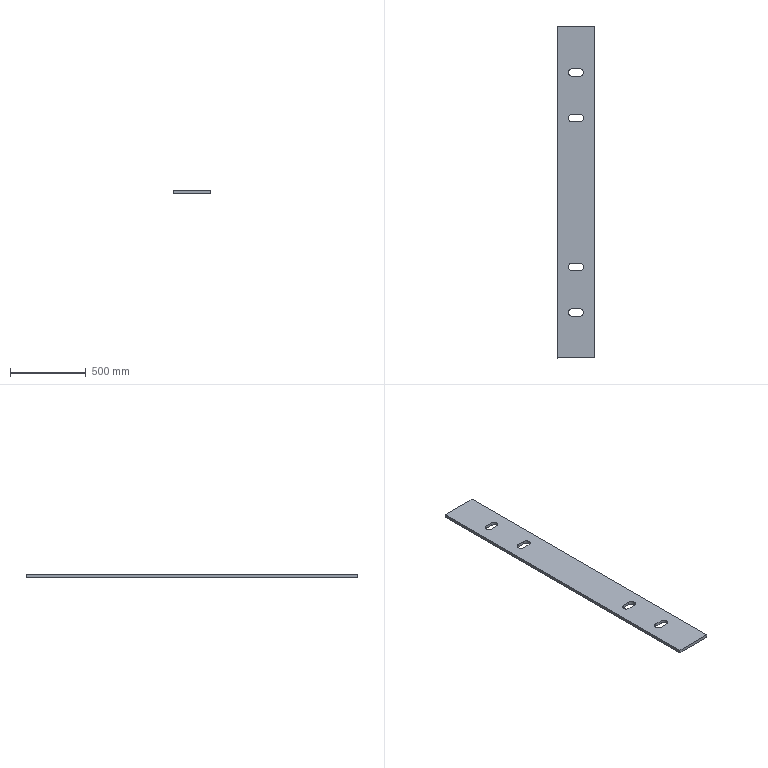Part | SolidWorks | features Extrusion 1 | 1 solid | 26 faces | box 250 x 2186 x 20 mm | volume 10572920 mm3 | plane 14 | cylinder 12 | commonest cylinder face diameters 50 x12
STEP:
#1=CARTESIAN_POINT('',(7508.99,4367.986,20.));
#2=VERTEX_POINT('',#1);
#3=CARTESIAN_POINT('',(7483.99,4342.986,20.));
#4=VERTEX_POINT('',#3);
#5=CARTESIAN_POINT('',(7508.99,4342.986,20.));
#6=DIRECTION('',(0.,0.,1.));
#7=DIRECTION('',(1.,0.,0.));
#8=AXIS2_PLACEMENT_3D('',#5,#6,#7);
#9=CIRCLE('',#8,25.);
#10=EDGE_CURVE('',#2,#4,#9,.T.);
#11=ORIENTED_EDGE('',*,*,#10,.T.);
#12=CARTESIAN_POINT('',(7483.99,4342.986,0.));
#13=VERTEX_POINT('',#12);
#14=CARTESIAN_POINT('',(7483.99,4342.986,20.));
#15=DIRECTION('',(0.,0.,-1.));
#16=VECTOR('',#15,1000.);
#17=LINE('',#14,#16);
#18=EDGE_CURVE('',#4,#13,#17,.T.);
#19=ORIENTED_EDGE('',*,*,#18,.T.);
#20=CARTESIAN_POINT('',(7508.99,4367.986,0.));
#21=VERTEX_POINT('',#20);
#22=CARTESIAN_POINT('',(7508.99,4342.986,0.));
#23=DIRECTION('',(0.,0.,1.));
#24=DIRECTION('',(1.,0.,0.));
#25=AXIS2_PLACEMENT_3D('',#22,#23,#24);
#26=CIRCLE('',#25,25.);
#27=EDGE_CURVE('',#21,#13,#26,.T.);
#28=ORIENTED_EDGE('',*,*,#27,.F.);
#29=CARTESIAN_POINT('',(7508.99,4367.986,20.));
#30=DIRECTION('',(0.,0.,-1.));
#31=VECTOR('',#30,1000.);
#32=LINE('',#29,#31);
#33=EDGE_CURVE('',#2,#21,#32,.T.);
#34=ORIENTED_EDGE('',*,*,#33,.F.);
#35=EDGE_LOOP('',(#11,#19,#28,#34));
#36=FACE_OUTER_BOUND('',#35,.T.);
#37=CARTESIAN_POINT('',(7508.99,4342.986,20.));
#38=DIRECTION('',(0.,0.,-1.));
#39=DIRECTION('',(-1.,0.,0.));
#40=AXIS2_PLACEMENT_3D('',#37,#38,#39);
#41=CYLINDRICAL_SURFACE('',#40,25.);
#42=ADVANCED_FACE('',(#36),#41,.F.);
#43=CARTESIAN_POINT('',(7508.99,4067.986,20.));
#44=VERTEX_POINT('',#43);
#45=CARTESIAN_POINT('',(7483.99,4042.986,20.));
#46=VERTEX_POINT('',#45);
#47=CARTESIAN_POINT('',(7508.99,4042.986,20.));
#48=DIRECTION('',(0.,0.,1.));
#49=DIRECTION('',(1.,0.,0.));
#50=AXIS2_PLACEMENT_3D('',#47,#48,#49);
#51=CIRCLE('',#50,25.);
#52=EDGE_CURVE('',#44,#46,#51,.T.);
#53=ORIENTED_EDGE('',*,*,#52,.T.);
#54=CARTESIAN_POINT('',(7483.99,4042.986,0.));
#55=VERTEX_POINT('',#54);
#56=CARTESIAN_POINT('',(7483.99,4042.986,20.));
#57=DIRECTION('',(0.,0.,-1.));
#58=VECTOR('',#57,1000.);
#59=LINE('',#56,#58);
#60=EDGE_CURVE('',#46,#55,#59,.T.);
#61=ORIENTED_EDGE('',*,*,#60,.T.);
#62=CARTESIAN_POINT('',(7508.99,4067.986,0.));
#63=VERTEX_POINT('',#62);
#64=CARTESIAN_POINT('',(7508.99,4042.986,0.));
#65=DIRECTION('',(0.,0.,1.));
#66=DIRECTION('',(1.,0.,0.));
#67=AXIS2_PLACEMENT_3D('',#64,#65,#66);
#68=CIRCLE('',#67,25.);
#69=EDGE_CURVE('',#63,#55,#68,.T.);
#70=ORIENTED_EDGE('',*,*,#69,.F.);
#71=CARTESIAN_POINT('',(7508.99,4067.986,20.));
#72=DIRECTION('',(0.,0.,-1.));
#73=VECTOR('',#72,1000.);
#74=LINE('',#71,#73);
#75=EDGE_CURVE('',#44,#63,#74,.T.);
#76=ORIENTED_EDGE('',*,*,#75,.F.);
#77=EDGE_LOOP('',(#53,#61,#70,#76));
#78=FACE_OUTER_BOUND('',#77,.T.);
#79=CARTESIAN_POINT('',(7508.99,4042.986,20.));
#80=DIRECTION('',(0.,0.,-1.));
#81=DIRECTION('',(-1.,0.,0.));
#82=AXIS2_PLACEMENT_3D('',#79,#80,#81);
#83=CYLINDRICAL_SURFACE('',#82,25.);
#84=ADVANCED_FACE('',(#78),#83,.F.);
#85=CARTESIAN_POINT('',(7508.99,3087.986,20.));
#86=VERTEX_POINT('',#85);
#87=CARTESIAN_POINT('',(7483.99,3062.986,20.));
#88=VERTEX_POINT('',#87);
#89=CARTESIAN_POINT('',(7508.99,3062.986,20.));
#90=DIRECTION('',(0.,0.,1.));
#91=DIRECTION('',(1.,0.,0.));
#92=AXIS2_PLACEMENT_3D('',#89,#90,#91);
#93=CIRCLE('',#92,25.);
#94=EDGE_CURVE('',#86,#88,#93,.T.);
#95=ORIENTED_EDGE('',*,*,#94,.T.);
#96=CARTESIAN_POINT('',(7483.99,3062.986,0.));
#97=VERTEX_POINT('',#96);
#98=CARTESIAN_POINT('',(7483.99,3062.986,20.));
#99=DIRECTION('',(0.,0.,-1.));
#100=VECTOR('',#99,1000.);
#101=LINE('',#98,#100);
#102=EDGE_CURVE('',#88,#97,#101,.T.);
#103=ORIENTED_EDGE('',*,*,#102,.T.);
#104=CARTESIAN_POINT('',(7508.99,3087.986,0.));
#105=VERTEX_POINT('',#104);
#106=CARTESIAN_POINT('',(7508.99,3062.986,0.));
#107=DIRECTION('',(0.,0.,1.));
#108=DIRECTION('',(1.,0.,0.));
#109=AXIS2_PLACEMENT_3D('',#106,#107,#108);
#110=CIRCLE('',#109,25.);
#111=EDGE_CURVE('',#105,#97,#110,.T.);
#112=ORIENTED_EDGE('',*,*,#111,.F.);
#113=CARTESIAN_POINT('',(7508.99,3087.986,20.));
#114=DIRECTION('',(0.,0.,-1.));
#115=VECTOR('',#114,1000.);
#116=LINE('',#113,#115);
#117=EDGE_CURVE('',#86,#105,#116,.T.);
#118=ORIENTED_EDGE('',*,*,#117,.F.);
#119=EDGE_LOOP('',(#95,#103,#112,#118));
#120=FACE_OUTER_BOUND('',#119,.T.);
#121=CARTESIAN_POINT('',(7508.99,3062.986,20.));
#122=DIRECTION('',(0.,0.,-1.));
#123=DIRECTION('',(-1.,0.,0.));
#124=AXIS2_PLACEMENT_3D('',#121,#122,#123);
#125=CYLINDRICAL_SURFACE('',#124,25.);
#126=ADVANCED_FACE('',(#120),#125,.F.);
#127=CARTESIAN_POINT('',(7508.99,2787.986,20.));
#128=VERTEX_POINT('',#127);
#129=CARTESIAN_POINT('',(7483.99,2762.986,20.));
#130=VERTEX_POINT('',#129);
#131=CARTESIAN_POINT('',(7508.99,2762.986,20.));
#132=DIRECTION('',(0.,0.,1.));
#133=DIRECTION('',(1.,0.,0.));
#134=AXIS2_PLACEMENT_3D('',#131,#132,#133);
#135=CIRCLE('',#134,25.);
#136=EDGE_CURVE('',#128,#130,#135,.T.);
#137=ORIENTED_EDGE('',*,*,#136,.T.);
#138=CARTESIAN_POINT('',(7483.99,2762.986,0.));
#139=VERTEX_POINT('',#138);
#140=CARTESIAN_POINT('',(7483.99,2762.986,20.));
#141=DIRECTION('',(0.,0.,-1.));
#142=VECTOR('',#141,1000.);
#143=LINE('',#140,#142);
#144=EDGE_CURVE('',#130,#139,#143,.T.);
#145=ORIENTED_EDGE('',*,*,#144,.T.);
#146=CARTESIAN_POINT('',(7508.99,2787.986,0.));
#147=VERTEX_POINT('',#146);
#148=CARTESIAN_POINT('',(7508.99,2762.986,0.));
#149=DIRECTION('',(0.,0.,1.));
#150=DIRECTION('',(1.,0.,0.));
#151=AXIS2_PLACEMENT_3D('',#148,#149,#150);
#152=CIRCLE('',#151,25.);
#153=EDGE_CURVE('',#147,#139,#152,.T.);
#154=ORIENTED_EDGE('',*,*,#153,.F.);
#155=CARTESIAN_POINT('',(7508.99,2787.986,20.));
#156=DIRECTION('',(0.,0.,-1.));
#157=VECTOR('',#156,1000.);
#158=LINE('',#155,#157);
#159=EDGE_CURVE('',#128,#147,#158,.T.);
#160=ORIENTED_EDGE('',*,*,#159,.F.);
#161=EDGE_LOOP('',(#137,#145,#154,#160));
#162=FACE_OUTER_BOUND('',#161,.T.);
#163=CARTESIAN_POINT('',(7508.99,2762.986,20.));
#164=DIRECTION('',(0.,0.,-1.));
#165=DIRECTION('',(-1.,0.,0.));
#166=AXIS2_PLACEMENT_3D('',#163,#164,#165);
#167=CYLINDRICAL_SURFACE('',#166,25.);
#168=ADVANCED_FACE('',(#162),#167,.F.);
#169=CARTESIAN_POINT('',(7408.99,2462.986,20.));
#170=VERTEX_POINT('',#169);
#171=CARTESIAN_POINT('',(7658.99,2462.986,20.));
#172=VERTEX_POINT('',#171);
#173=CARTESIAN_POINT('',(7408.99,2462.986,20.));
#174=DIRECTION('',(1.,0.,0.));
#175=VECTOR('',#174,1000.);
#176=LINE('',#173,#175);
#177=EDGE_CURVE('',#170,#172,#176,.T.);
#178=ORIENTED_EDGE('',*,*,#177,.T.);
#179=CARTESIAN_POINT('',(7658.99,4648.986,20.));
#180=VERTEX_POINT('',#179);
#181=CARTESIAN_POINT('',(7658.99,2462.986,20.));
#182=DIRECTION('',(0.,1.,0.));
#183=VECTOR('',#182,1000.);
#184=LINE('',#181,#183);
#185=EDGE_CURVE('',#172,#180,#184,.T.);
#186=ORIENTED_EDGE('',*,*,#185,.T.);
#187=CARTESIAN_POINT('',(7408.99,4648.986,20.));
#188=VERTEX_POINT('',#187);
#189=CARTESIAN_POINT('',(7408.99,4648.986,20.));
#190=DIRECTION('',(-1.,0.,0.));
#191=VECTOR('',#190,1000.);
#192=LINE('',#189,#191);
#193=EDGE_CURVE('',#180,#188,#192,.T.);
#194=ORIENTED_EDGE('',*,*,#193,.T.);
#195=CARTESIAN_POINT('',(7408.99,2462.986,20.));
#196=DIRECTION('',(0.,-1.,0.));
#197=VECTOR('',#196,1000.);
#198=LINE('',#195,#197);
#199=EDGE_CURVE('',#188,#170,#198,.T.);
#200=ORIENTED_EDGE('',*,*,#199,.T.);
#201=EDGE_LOOP('',(#178,#186,#194,#200));
#202=FACE_OUTER_BOUND('',#201,.T.);
#203=CARTESIAN_POINT('',(7508.99,2737.986,20.));
#204=VERTEX_POINT('',#203);
#205=CARTESIAN_POINT('',(7558.99,2737.986,20.));
#206=VERTEX_POINT('',#205);
#207=CARTESIAN_POINT('',(7508.99,2737.986,20.));
#208=DIRECTION('',(1.,0.,0.));
#209=VECTOR('',#208,1000.);
#210=LINE('',#207,#209);
#211=EDGE_CURVE('',#204,#206,#210,.T.);
#212=ORIENTED_EDGE('',*,*,#211,.F.);
#213=CARTESIAN_POINT('',(7508.99,2762.986,20.));
#214=DIRECTION('',(0.,0.,1.));
#215=DIRECTION('',(1.,0.,0.));
#216=AXIS2_PLACEMENT_3D('',#213,#214,#215);
#217=CIRCLE('',#216,25.);
#218=EDGE_CURVE('',#130,#204,#217,.T.);
#219=ORIENTED_EDGE('',*,*,#218,.F.);
#220=ORIENTED_EDGE('',*,*,#136,.F.);
#221=CARTESIAN_POINT('',(7558.989,2787.986,20.));
#222=VERTEX_POINT('',#221);
#223=CARTESIAN_POINT('',(7508.99,2787.986,20.));
#224=DIRECTION('',(-1.,0.,0.));
#225=VECTOR('',#224,1000.);
#226=LINE('',#223,#225);
#227=EDGE_CURVE('',#222,#128,#226,.T.);
#228=ORIENTED_EDGE('',*,*,#227,.F.);
#229=CARTESIAN_POINT('',(7558.99,2762.986,20.));
#230=DIRECTION('',(0.,0.,1.));
#231=DIRECTION('',(1.,0.,0.));
#232=AXIS2_PLACEMENT_3D('',#229,#230,#231);
#233=CIRCLE('',#232,25.);
#234=EDGE_CURVE('',#206,#222,#233,.T.);
#235=ORIENTED_EDGE('',*,*,#234,.F.);
#236=EDGE_LOOP('',(#212,#219,#220,#228,#235));
#237=FACE_BOUND('',#236,.T.);
#238=CARTESIAN_POINT('',(7508.99,3037.986,20.));
#239=VERTEX_POINT('',#238);
#240=CARTESIAN_POINT('',(7558.99,3037.986,20.));
#241=VERTEX_POINT('',#240);
#242=CARTESIAN_POINT('',(7558.99,3037.986,20.));
#243=DIRECTION('',(1.,0.,0.));
#244=VECTOR('',#243,1000.);
#245=LINE('',#242,#244);
#246=EDGE_CURVE('',#239,#241,#245,.T.);
#247=ORIENTED_EDGE('',*,*,#246,.F.);
#248=CARTESIAN_POINT('',(7508.99,3062.986,20.));
#249=DIRECTION('',(0.,0.,1.));
#250=DIRECTION('',(1.,0.,0.));
#251=AXIS2_PLACEMENT_3D('',#248,#249,#250);
#252=CIRCLE('',#251,25.);
#253=EDGE_CURVE('',#88,#239,#252,.T.);
#254=ORIENTED_EDGE('',*,*,#253,.F.);
#255=ORIENTED_EDGE('',*,*,#94,.F.);
#256=CARTESIAN_POINT('',(7558.989,3087.986,20.));
#257=VERTEX_POINT('',#256);
#258=CARTESIAN_POINT('',(7508.99,3087.986,20.));
#259=DIRECTION('',(-1.,0.,0.));
#260=VECTOR('',#259,1000.);
#261=LINE('',#258,#260);
#262=EDGE_CURVE('',#257,#86,#261,.T.);
#263=ORIENTED_EDGE('',*,*,#262,.F.);
#264=CARTESIAN_POINT('',(7558.99,3062.986,20.));
#265=DIRECTION('',(0.,0.,1.));
#266=DIRECTION('',(1.,0.,0.));
#267=AXIS2_PLACEMENT_3D('',#264,#265,#266);
#268=CIRCLE('',#267,25.);
#269=EDGE_CURVE('',#241,#257,#268,.T.);
#270=ORIENTED_EDGE('',*,*,#269,.F.);
#271=EDGE_LOOP('',(#247,#254,#255,#263,#270));
#272=FACE_BOUND('',#271,.T.);
#273=CARTESIAN_POINT('',(7508.99,4017.986,20.));
#274=VERTEX_POINT('',#273);
#275=CARTESIAN_POINT('',(7558.99,4017.986,20.));
#276=VERTEX_POINT('',#275);
#277=CARTESIAN_POINT('',(7508.99,4017.986,20.));
#278=DIRECTION('',(1.,0.,0.));
#279=VECTOR('',#278,1000.);
#280=LINE('',#277,#279);
#281=EDGE_CURVE('',#274,#276,#280,.T.);
#282=ORIENTED_EDGE('',*,*,#281,.F.);
#283=CARTESIAN_POINT('',(7508.99,4042.986,20.));
#284=DIRECTION('',(0.,0.,1.));
#285=DIRECTION('',(1.,0.,0.));
#286=AXIS2_PLACEMENT_3D('',#283,#284,#285);
#287=CIRCLE('',#286,25.);
#288=EDGE_CURVE('',#46,#274,#287,.T.);
#289=ORIENTED_EDGE('',*,*,#288,.F.);
#290=ORIENTED_EDGE('',*,*,#52,.F.);
#291=CARTESIAN_POINT('',(7558.99,4067.986,20.));
#292=VERTEX_POINT('',#291);
#293=CARTESIAN_POINT('',(7508.99,4067.986,20.));
#294=DIRECTION('',(-1.,0.,0.));
#295=VECTOR('',#294,1000.);
#296=LINE('',#293,#295);
#297=EDGE_CURVE('',#292,#44,#296,.T.);
#298=ORIENTED_EDGE('',*,*,#297,.F.);
#299=CARTESIAN_POINT('',(7558.99,4042.986,20.));
#300=DIRECTION('',(0.,0.,1.));
#301=DIRECTION('',(1.,0.,0.));
#302=AXIS2_PLACEMENT_3D('',#299,#300,#301);
#303=CIRCLE('',#302,25.);
#304=EDGE_CURVE('',#276,#292,#303,.T.);
#305=ORIENTED_EDGE('',*,*,#304,.F.);
#306=EDGE_LOOP('',(#282,#289,#290,#298,#305));
#307=FACE_BOUND('',#306,.T.);
#308=CARTESIAN_POINT('',(7508.99,4317.986,20.));
#309=VERTEX_POINT('',#308);
#310=CARTESIAN_POINT('',(7558.99,4317.986,20.));
#311=VERTEX_POINT('',#310);
#312=CARTESIAN_POINT('',(7508.99,4317.986,20.));
#313=DIRECTION('',(1.,0.,0.));
#314=VECTOR('',#313,1000.);
#315=LINE('',#312,#314);
#316=EDGE_CURVE('',#309,#311,#315,.T.);
#317=ORIENTED_EDGE('',*,*,#316,.F.);
#318=CARTESIAN_POINT('',(7508.99,4342.986,20.));
#319=DIRECTION('',(0.,0.,1.));
#320=DIRECTION('',(1.,0.,0.));
#321=AXIS2_PLACEMENT_3D('',#318,#319,#320);
#322=CIRCLE('',#321,25.);
#323=EDGE_CURVE('',#4,#309,#322,.T.);
#324=ORIENTED_EDGE('',*,*,#323,.F.);
#325=ORIENTED_EDGE('',*,*,#10,.F.);
#326=CARTESIAN_POINT('',(7558.99,4367.986,20.));
#327=VERTEX_POINT('',#326);
#328=CARTESIAN_POINT('',(7508.99,4367.986,20.));
#329=DIRECTION('',(-1.,0.,0.));
#330=VECTOR('',#329,1000.);
#331=LINE('',#328,#330);
#332=EDGE_CURVE('',#327,#2,#331,.T.);
#333=ORIENTED_EDGE('',*,*,#332,.F.);
#334=CARTESIAN_POINT('',(7558.99,4342.986,20.));
#335=DIRECTION('',(0.,0.,1.));
#336=DIRECTION('',(1.,0.,0.));
#337=AXIS2_PLACEMENT_3D('',#334,#335,#336);
#338=CIRCLE('',#337,25.);
#339=EDGE_CURVE('',#311,#327,#338,.T.);
#340=ORIENTED_EDGE('',*,*,#339,.F.);
#341=EDGE_LOOP('',(#317,#324,#325,#333,#340));
#342=FACE_BOUND('',#341,.T.);
#343=CARTESIAN_POINT('',(0.,0.,20.));
#344=DIRECTION('',(0.,0.,1.));
#345=DIRECTION('',(1.,0.,0.));
#346=AXIS2_PLACEMENT_3D('',#343,#344,#345);
#347=PLANE('',#346);
#348=ADVANCED_FACE('',(#202,#237,#272,#307,#342),#347,.T.);
#349=ORIENTED_EDGE('',*,*,#69,.T.);
#350=CARTESIAN_POINT('',(7508.99,4017.986,0.));
#351=VERTEX_POINT('',#350);
#352=CARTESIAN_POINT('',(7508.99,4042.986,0.));
#353=DIRECTION('',(0.,0.,1.));
#354=DIRECTION('',(1.,0.,0.));
#355=AXIS2_PLACEMENT_3D('',#352,#353,#354);
#356=CIRCLE('',#355,25.);
#357=EDGE_CURVE('',#55,#351,#356,.T.);
#358=ORIENTED_EDGE('',*,*,#357,.T.);
#359=CARTESIAN_POINT('',(7558.99,4017.986,0.));
#360=VERTEX_POINT('',#359);
#361=CARTESIAN_POINT('',(7508.99,4017.986,0.));
#362=DIRECTION('',(1.,0.,0.));
#363=VECTOR('',#362,1000.);
#364=LINE('',#361,#363);
#365=EDGE_CURVE('',#351,#360,#364,.T.);
#366=ORIENTED_EDGE('',*,*,#365,.T.);
#367=CARTESIAN_POINT('',(7558.99,4067.986,0.));
#368=VERTEX_POINT('',#367);
#369=CARTESIAN_POINT('',(7558.99,4042.986,0.));
#370=DIRECTION('',(0.,0.,1.));
#371=DIRECTION('',(1.,0.,0.));
#372=AXIS2_PLACEMENT_3D('',#369,#370,#371);
#373=CIRCLE('',#372,25.);
#374=EDGE_CURVE('',#360,#368,#373,.T.);
#375=ORIENTED_EDGE('',*,*,#374,.T.);
#376=CARTESIAN_POINT('',(7508.99,4067.986,0.));
#377=DIRECTION('',(-1.,0.,0.));
#378=VECTOR('',#377,1000.);
#379=LINE('',#376,#378);
#380=EDGE_CURVE('',#368,#63,#379,.T.);
#381=ORIENTED_EDGE('',*,*,#380,.T.);
#382=EDGE_LOOP('',(#349,#358,#366,#375,#381));
#383=FACE_BOUND('',#382,.T.);
#384=ORIENTED_EDGE('',*,*,#153,.T.);
#385=CARTESIAN_POINT('',(7508.99,2737.986,0.));
#386=VERTEX_POINT('',#385);
#387=CARTESIAN_POINT('',(7508.99,2762.986,0.));
#388=DIRECTION('',(0.,0.,1.));
#389=DIRECTION('',(1.,0.,0.));
#390=AXIS2_PLACEMENT_3D('',#387,#388,#389);
#391=CIRCLE('',#390,25.);
#392=EDGE_CURVE('',#139,#386,#391,.T.);
#393=ORIENTED_EDGE('',*,*,#392,.T.);
#394=CARTESIAN_POINT('',(7558.99,2737.986,0.));
#395=VERTEX_POINT('',#394);
#396=CARTESIAN_POINT('',(7508.99,2737.986,0.));
#397=DIRECTION('',(1.,0.,0.));
#398=VECTOR('',#397,1000.);
#399=LINE('',#396,#398);
#400=EDGE_CURVE('',#386,#395,#399,.T.);
#401=ORIENTED_EDGE('',*,*,#400,.T.);
#402=CARTESIAN_POINT('',(7558.989,2787.986,0.));
#403=VERTEX_POINT('',#402);
#404=CARTESIAN_POINT('',(7558.99,2762.986,0.));
#405=DIRECTION('',(0.,0.,1.));
#406=DIRECTION('',(1.,0.,0.));
#407=AXIS2_PLACEMENT_3D('',#404,#405,#406);
#408=CIRCLE('',#407,25.);
#409=EDGE_CURVE('',#395,#403,#408,.T.);
#410=ORIENTED_EDGE('',*,*,#409,.T.);
#411=CARTESIAN_POINT('',(7508.99,2787.986,0.));
#412=DIRECTION('',(-1.,0.,0.));
#413=VECTOR('',#412,1000.);
#414=LINE('',#411,#413);
#415=EDGE_CURVE('',#403,#147,#414,.T.);
#416=ORIENTED_EDGE('',*,*,#415,.T.);
#417=EDGE_LOOP('',(#384,#393,#401,#410,#416));
#418=FACE_BOUND('',#417,.T.);
#419=CARTESIAN_POINT('',(7408.99,2462.986,0.));
#420=VERTEX_POINT('',#419);
#421=CARTESIAN_POINT('',(7658.99,2462.986,0.));
#422=VERTEX_POINT('',#421);
#423=CARTESIAN_POINT('',(7408.99,2462.986,0.));
#424=DIRECTION('',(1.,0.,0.));
#425=VECTOR('',#424,1000.);
#426=LINE('',#423,#425);
#427=EDGE_CURVE('',#420,#422,#426,.T.);
#428=ORIENTED_EDGE('',*,*,#427,.F.);
#429=CARTESIAN_POINT('',(7408.99,4648.986,0.));
#430=VERTEX_POINT('',#429);
#431=CARTESIAN_POINT('',(7408.99,2462.986,0.));
#432=DIRECTION('',(0.,-1.,0.));
#433=VECTOR('',#432,1000.);
#434=LINE('',#431,#433);
#435=EDGE_CURVE('',#430,#420,#434,.T.);
#436=ORIENTED_EDGE('',*,*,#435,.F.);
#437=CARTESIAN_POINT('',(7658.99,4648.986,0.));
#438=VERTEX_POINT('',#437);
#439=CARTESIAN_POINT('',(7408.99,4648.986,0.));
#440=DIRECTION('',(-1.,0.,0.));
#441=VECTOR('',#440,1000.);
#442=LINE('',#439,#441);
#443=EDGE_CURVE('',#438,#430,#442,.T.);
#444=ORIENTED_EDGE('',*,*,#443,.F.);
#445=CARTESIAN_POINT('',(7658.99,2462.986,0.));
#446=DIRECTION('',(0.,1.,0.));
#447=VECTOR('',#446,1000.);
#448=LINE('',#445,#447);
#449=EDGE_CURVE('',#422,#438,#448,.T.);
#450=ORIENTED_EDGE('',*,*,#449,.F.);
#451=EDGE_LOOP('',(#428,#436,#444,#450));
#452=FACE_OUTER_BOUND('',#451,.T.);
#453=ORIENTED_EDGE('',*,*,#111,.T.);
#454=CARTESIAN_POINT('',(7508.99,3037.986,0.));
#455=VERTEX_POINT('',#454);
#456=CARTESIAN_POINT('',(7508.99,3062.986,0.));
#457=DIRECTION('',(0.,0.,1.));
#458=DIRECTION('',(1.,0.,0.));
#459=AXIS2_PLACEMENT_3D('',#456,#457,#458);
#460=CIRCLE('',#459,25.);
#461=EDGE_CURVE('',#97,#455,#460,.T.);
#462=ORIENTED_EDGE('',*,*,#461,.T.);
#463=CARTESIAN_POINT('',(7558.99,3037.986,0.));
#464=VERTEX_POINT('',#463);
#465=CARTESIAN_POINT('',(7558.99,3037.986,0.));
#466=DIRECTION('',(1.,0.,0.));
#467=VECTOR('',#466,1000.);
#468=LINE('',#465,#467);
#469=EDGE_CURVE('',#455,#464,#468,.T.);
#470=ORIENTED_EDGE('',*,*,#469,.T.);
#471=CARTESIAN_POINT('',(7558.989,3087.986,0.));
#472=VERTEX_POINT('',#471);
#473=CARTESIAN_POINT('',(7558.99,3062.986,0.));
#474=DIRECTION('',(0.,0.,1.));
#475=DIRECTION('',(1.,0.,0.));
#476=AXIS2_PLACEMENT_3D('',#473,#474,#475);
#477=CIRCLE('',#476,25.);
#478=EDGE_CURVE('',#464,#472,#477,.T.);
#479=ORIENTED_EDGE('',*,*,#478,.T.);
#480=CARTESIAN_POINT('',(7508.99,3087.986,0.));
#481=DIRECTION('',(-1.,0.,0.));
#482=VECTOR('',#481,1000.);
#483=LINE('',#480,#482);
#484=EDGE_CURVE('',#472,#105,#483,.T.);
#485=ORIENTED_EDGE('',*,*,#484,.T.);
#486=EDGE_LOOP('',(#453,#462,#470,#479,#485));
#487=FACE_BOUND('',#486,.T.);
#488=ORIENTED_EDGE('',*,*,#27,.T.);
#489=CARTESIAN_POINT('',(7508.99,4317.986,0.));
#490=VERTEX_POINT('',#489);
#491=CARTESIAN_POINT('',(7508.99,4342.986,0.));
#492=DIRECTION('',(0.,0.,1.));
#493=DIRECTION('',(1.,0.,0.));
#494=AXIS2_PLACEMENT_3D('',#491,#492,#493);
#495=CIRCLE('',#494,25.);
#496=EDGE_CURVE('',#13,#490,#495,.T.);
#497=ORIENTED_EDGE('',*,*,#496,.T.);
#498=CARTESIAN_POINT('',(7558.99,4317.986,0.));
#499=VERTEX_POINT('',#498);
#500=CARTESIAN_POINT('',(7508.99,4317.986,0.));
#501=DIRECTION('',(1.,0.,0.));
#502=VECTOR('',#501,1000.);
#503=LINE('',#500,#502);
#504=EDGE_CURVE('',#490,#499,#503,.T.);
#505=ORIENTED_EDGE('',*,*,#504,.T.);
#506=CARTESIAN_POINT('',(7558.99,4367.986,0.));
#507=VERTEX_POINT('',#506);
#508=CARTESIAN_POINT('',(7558.99,4342.986,0.));
#509=DIRECTION('',(0.,0.,1.));
#510=DIRECTION('',(1.,0.,0.));
#511=AXIS2_PLACEMENT_3D('',#508,#509,#510);
#512=CIRCLE('',#511,25.);
#513=EDGE_CURVE('',#499,#507,#512,.T.);
#514=ORIENTED_EDGE('',*,*,#513,.T.);
#515=CARTESIAN_POINT('',(7508.99,4367.986,0.));
#516=DIRECTION('',(-1.,0.,0.));
#517=VECTOR('',#516,1000.);
#518=LINE('',#515,#517);
#519=EDGE_CURVE('',#507,#21,#518,.T.);
#520=ORIENTED_EDGE('',*,*,#519,.T.);
#521=EDGE_LOOP('',(#488,#497,#505,#514,#520));
#522=FACE_BOUND('',#521,.T.);
#523=CARTESIAN_POINT('',(0.,0.,0.));
#524=DIRECTION('',(0.,0.,1.));
#525=DIRECTION('',(1.,0.,0.));
#526=AXIS2_PLACEMENT_3D('',#523,#524,#525);
#527=PLANE('',#526);
#528=ADVANCED_FACE('',(#383,#418,#452,#487,#522),#527,.F.);
#529=ORIENTED_EDGE('',*,*,#427,.T.);
#530=CARTESIAN_POINT('',(7658.99,2462.986,20.));
#531=DIRECTION('',(0.,0.,-1.));
#532=VECTOR('',#531,1000.);
#533=LINE('',#530,#532);
#534=EDGE_CURVE('',#172,#422,#533,.T.);
#535=ORIENTED_EDGE('',*,*,#534,.F.);
#536=ORIENTED_EDGE('',*,*,#177,.F.);
#537=CARTESIAN_POINT('',(7408.99,2462.986,20.));
#538=DIRECTION('',(0.,0.,-1.));
#539=VECTOR('',#538,1000.);
#540=LINE('',#537,#539);
#541=EDGE_CURVE('',#170,#420,#540,.T.);
#542=ORIENTED_EDGE('',*,*,#541,.T.);
#543=EDGE_LOOP('',(#529,#535,#536,#542));
#544=FACE_OUTER_BOUND('',#543,.T.);
#545=CARTESIAN_POINT('',(7408.99,2462.986,20.));
#546=DIRECTION('',(0.,1.,0.));
#547=DIRECTION('',(-1.,0.,0.));
#548=AXIS2_PLACEMENT_3D('',#545,#546,#547);
#549=PLANE('',#548);
#550=ADVANCED_FACE('',(#544),#549,.F.);
#551=ORIENTED_EDGE('',*,*,#449,.T.);
#552=CARTESIAN_POINT('',(7658.99,4648.986,20.));
#553=DIRECTION('',(0.,0.,-1.));
#554=VECTOR('',#553,1000.);
#555=LINE('',#552,#554);
#556=EDGE_CURVE('',#180,#438,#555,.T.);
#557=ORIENTED_EDGE('',*,*,#556,.F.);
#558=ORIENTED_EDGE('',*,*,#185,.F.);
#559=ORIENTED_EDGE('',*,*,#534,.T.);
#560=EDGE_LOOP('',(#551,#557,#558,#559));
#561=FACE_OUTER_BOUND('',#560,.T.);
#562=CARTESIAN_POINT('',(7658.99,2462.986,20.));
#563=DIRECTION('',(-1.,0.,0.));
#564=DIRECTION('',(0.,0.,1.));
#565=AXIS2_PLACEMENT_3D('',#562,#563,#564);
#566=PLANE('',#565);
#567=ADVANCED_FACE('',(#561),#566,.F.);
#568=ORIENTED_EDGE('',*,*,#443,.T.);
#569=CARTESIAN_POINT('',(7408.99,4648.986,20.));
#570=DIRECTION('',(0.,0.,-1.));
#571=VECTOR('',#570,1000.);
#572=LINE('',#569,#571);
#573=EDGE_CURVE('',#188,#430,#572,.T.);
#574=ORIENTED_EDGE('',*,*,#573,.F.);
#575=ORIENTED_EDGE('',*,*,#193,.F.);
#576=ORIENTED_EDGE('',*,*,#556,.T.);
#577=EDGE_LOOP('',(#568,#574,#575,#576));
#578=FACE_OUTER_BOUND('',#577,.T.);
#579=CARTESIAN_POINT('',(7408.99,4648.986,20.));
#580=DIRECTION('',(0.,-1.,0.));
#581=DIRECTION('',(0.,0.,-1.));
#582=AXIS2_PLACEMENT_3D('',#579,#580,#581);
#583=PLANE('',#582);
#584=ADVANCED_FACE('',(#578),#583,.F.);
#585=ORIENTED_EDGE('',*,*,#435,.T.);
#586=ORIENTED_EDGE('',*,*,#541,.F.);
#587=ORIENTED_EDGE('',*,*,#199,.F.);
#588=ORIENTED_EDGE('',*,*,#573,.T.);
#589=EDGE_LOOP('',(#585,#586,#587,#588));
#590=FACE_OUTER_BOUND('',#589,.T.);
#591=CARTESIAN_POINT('',(7408.99,2462.986,20.));
#592=DIRECTION('',(1.,0.,0.));
#593=DIRECTION('',(0.,1.,0.));
#594=AXIS2_PLACEMENT_3D('',#591,#592,#593);
#595=PLANE('',#594);
#596=ADVANCED_FACE('',(#590),#595,.F.);
#597=ORIENTED_EDGE('',*,*,#144,.F.);
#598=ORIENTED_EDGE('',*,*,#218,.T.);
#599=CARTESIAN_POINT('',(7508.99,2737.986,20.));
#600=DIRECTION('',(0.,0.,-1.));
#601=VECTOR('',#600,1000.);
#602=LINE('',#599,#601);
#603=EDGE_CURVE('',#204,#386,#602,.T.);
#604=ORIENTED_EDGE('',*,*,#603,.T.);
#605=ORIENTED_EDGE('',*,*,#392,.F.);
#606=EDGE_LOOP('',(#597,#598,#604,#605));
#607=FACE_OUTER_BOUND('',#606,.T.);
#608=CARTESIAN_POINT('',(7508.99,2762.986,20.));
#609=DIRECTION('',(0.,0.,-1.));
#610=DIRECTION('',(-1.,0.,0.));
#611=AXIS2_PLACEMENT_3D('',#608,#609,#610);
#612=CYLINDRICAL_SURFACE('',#611,25.);
#613=ADVANCED_FACE('',(#607),#612,.F.);
#614=ORIENTED_EDGE('',*,*,#400,.F.);
#615=ORIENTED_EDGE('',*,*,#603,.F.);
#616=ORIENTED_EDGE('',*,*,#211,.T.);
#617=CARTESIAN_POINT('',(7558.99,2737.986,20.));
#618=DIRECTION('',(0.,0.,-1.));
#619=VECTOR('',#618,1000.);
#620=LINE('',#617,#619);
#621=EDGE_CURVE('',#206,#395,#620,.T.);
#622=ORIENTED_EDGE('',*,*,#621,.T.);
#623=EDGE_LOOP('',(#614,#615,#616,#622));
#624=FACE_OUTER_BOUND('',#623,.T.);
#625=CARTESIAN_POINT('',(7508.99,2737.986,20.));
#626=DIRECTION('',(0.,1.,0.));
#627=DIRECTION('',(0.,0.,1.));
#628=AXIS2_PLACEMENT_3D('',#625,#626,#627);
#629=PLANE('',#628);
#630=ADVANCED_FACE('',(#624),#629,.T.);
#631=ORIENTED_EDGE('',*,*,#409,.F.);
#632=ORIENTED_EDGE('',*,*,#621,.F.);
#633=ORIENTED_EDGE('',*,*,#234,.T.);
#634=CARTESIAN_POINT('',(7558.989,2787.986,20.));
#635=DIRECTION('',(0.,0.,-1.));
#636=VECTOR('',#635,1000.);
#637=LINE('',#634,#636);
#638=EDGE_CURVE('',#222,#403,#637,.T.);
#639=ORIENTED_EDGE('',*,*,#638,.T.);
#640=EDGE_LOOP('',(#631,#632,#633,#639));
#641=FACE_OUTER_BOUND('',#640,.T.);
#642=CARTESIAN_POINT('',(7558.99,2762.986,20.));
#643=DIRECTION('',(0.,0.,-1.));
#644=DIRECTION('',(-1.,0.,0.));
#645=AXIS2_PLACEMENT_3D('',#642,#643,#644);
#646=CYLINDRICAL_SURFACE('',#645,25.);
#647=ADVANCED_FACE('',(#641),#646,.F.);
#648=ORIENTED_EDGE('',*,*,#415,.F.);
#649=ORIENTED_EDGE('',*,*,#638,.F.);
#650=ORIENTED_EDGE('',*,*,#227,.T.);
#651=ORIENTED_EDGE('',*,*,#159,.T.);
#652=EDGE_LOOP('',(#648,#649,#650,#651));
#653=FACE_OUTER_BOUND('',#652,.T.);
#654=CARTESIAN_POINT('',(7508.99,2787.986,20.));
#655=DIRECTION('',(0.,-1.,0.));
#656=DIRECTION('',(0.,0.,-1.));
#657=AXIS2_PLACEMENT_3D('',#654,#655,#656);
#658=PLANE('',#657);
#659=ADVANCED_FACE('',(#653),#658,.T.);
#660=ORIENTED_EDGE('',*,*,#102,.F.);
#661=ORIENTED_EDGE('',*,*,#253,.T.);
#662=CARTESIAN_POINT('',(7508.99,3037.986,20.));
#663=DIRECTION('',(0.,0.,-1.));
#664=VECTOR('',#663,1000.);
#665=LINE('',#662,#664);
#666=EDGE_CURVE('',#239,#455,#665,.T.);
#667=ORIENTED_EDGE('',*,*,#666,.T.);
#668=ORIENTED_EDGE('',*,*,#461,.F.);
#669=EDGE_LOOP('',(#660,#661,#667,#668));
#670=FACE_OUTER_BOUND('',#669,.T.);
#671=CARTESIAN_POINT('',(7508.99,3062.986,20.));
#672=DIRECTION('',(0.,0.,-1.));
#673=DIRECTION('',(-1.,0.,0.));
#674=AXIS2_PLACEMENT_3D('',#671,#672,#673);
#675=CYLINDRICAL_SURFACE('',#674,25.);
#676=ADVANCED_FACE('',(#670),#675,.F.);
#677=ORIENTED_EDGE('',*,*,#469,.F.);
#678=ORIENTED_EDGE('',*,*,#666,.F.);
#679=ORIENTED_EDGE('',*,*,#246,.T.);
#680=CARTESIAN_POINT('',(7558.99,3037.986,20.));
#681=DIRECTION('',(0.,0.,-1.));
#682=VECTOR('',#681,1000.);
#683=LINE('',#680,#682);
#684=EDGE_CURVE('',#241,#464,#683,.T.);
#685=ORIENTED_EDGE('',*,*,#684,.T.);
#686=EDGE_LOOP('',(#677,#678,#679,#685));
#687=FACE_OUTER_BOUND('',#686,.T.);
#688=CARTESIAN_POINT('',(7558.99,3037.986,20.));
#689=DIRECTION('',(0.,1.,0.));
#690=DIRECTION('',(0.,0.,1.));
#691=AXIS2_PLACEMENT_3D('',#688,#689,#690);
#692=PLANE('',#691);
#693=ADVANCED_FACE('',(#687),#692,.T.);
#694=ORIENTED_EDGE('',*,*,#478,.F.);
#695=ORIENTED_EDGE('',*,*,#684,.F.);
#696=ORIENTED_EDGE('',*,*,#269,.T.);
#697=CARTESIAN_POINT('',(7558.989,3087.986,20.));
#698=DIRECTION('',(0.,0.,-1.));
#699=VECTOR('',#698,1000.);
#700=LINE('',#697,#699);
#701=EDGE_CURVE('',#257,#472,#700,.T.);
#702=ORIENTED_EDGE('',*,*,#701,.T.);
#703=EDGE_LOOP('',(#694,#695,#696,#702));
#704=FACE_OUTER_BOUND('',#703,.T.);
#705=CARTESIAN_POINT('',(7558.99,3062.986,20.));
#706=DIRECTION('',(0.,0.,-1.));
#707=DIRECTION('',(-1.,0.,0.));
#708=AXIS2_PLACEMENT_3D('',#705,#706,#707);
#709=CYLINDRICAL_SURFACE('',#708,25.);
#710=ADVANCED_FACE('',(#704),#709,.F.);
#711=ORIENTED_EDGE('',*,*,#484,.F.);
#712=ORIENTED_EDGE('',*,*,#701,.F.);
#713=ORIENTED_EDGE('',*,*,#262,.T.);
#714=ORIENTED_EDGE('',*,*,#117,.T.);
#715=EDGE_LOOP('',(#711,#712,#713,#714));
#716=FACE_OUTER_BOUND('',#715,.T.);
#717=CARTESIAN_POINT('',(7508.99,3087.986,20.));
#718=DIRECTION('',(0.,-1.,0.));
#719=DIRECTION('',(0.,0.,-1.));
#720=AXIS2_PLACEMENT_3D('',#717,#718,#719);
#721=PLANE('',#720);
#722=ADVANCED_FACE('',(#716),#721,.T.);
#723=ORIENTED_EDGE('',*,*,#60,.F.);
#724=ORIENTED_EDGE('',*,*,#288,.T.);
#725=CARTESIAN_POINT('',(7508.99,4017.986,20.));
#726=DIRECTION('',(0.,0.,-1.));
#727=VECTOR('',#726,1000.);
#728=LINE('',#725,#727);
#729=EDGE_CURVE('',#274,#351,#728,.T.);
#730=ORIENTED_EDGE('',*,*,#729,.T.);
#731=ORIENTED_EDGE('',*,*,#357,.F.);
#732=EDGE_LOOP('',(#723,#724,#730,#731));
#733=FACE_OUTER_BOUND('',#732,.T.);
#734=CARTESIAN_POINT('',(7508.99,4042.986,20.));
#735=DIRECTION('',(0.,0.,-1.));
#736=DIRECTION('',(-1.,0.,0.));
#737=AXIS2_PLACEMENT_3D('',#734,#735,#736);
#738=CYLINDRICAL_SURFACE('',#737,25.);
#739=ADVANCED_FACE('',(#733),#738,.F.);
#740=ORIENTED_EDGE('',*,*,#365,.F.);
#741=ORIENTED_EDGE('',*,*,#729,.F.);
#742=ORIENTED_EDGE('',*,*,#281,.T.);
#743=CARTESIAN_POINT('',(7558.99,4017.986,20.));
#744=DIRECTION('',(0.,0.,-1.));
#745=VECTOR('',#744,1000.);
#746=LINE('',#743,#745);
#747=EDGE_CURVE('',#276,#360,#746,.T.);
#748=ORIENTED_EDGE('',*,*,#747,.T.);
#749=EDGE_LOOP('',(#740,#741,#742,#748));
#750=FACE_OUTER_BOUND('',#749,.T.);
#751=CARTESIAN_POINT('',(7508.99,4017.986,20.));
#752=DIRECTION('',(0.,1.,0.));
#753=DIRECTION('',(0.,0.,1.));
#754=AXIS2_PLACEMENT_3D('',#751,#752,#753);
#755=PLANE('',#754);
#756=ADVANCED_FACE('',(#750),#755,.T.);
#757=ORIENTED_EDGE('',*,*,#374,.F.);
#758=ORIENTED_EDGE('',*,*,#747,.F.);
#759=ORIENTED_EDGE('',*,*,#304,.T.);
#760=CARTESIAN_POINT('',(7558.99,4067.986,20.));
#761=DIRECTION('',(0.,0.,-1.));
#762=VECTOR('',#761,1000.);
#763=LINE('',#760,#762);
#764=EDGE_CURVE('',#292,#368,#763,.T.);
#765=ORIENTED_EDGE('',*,*,#764,.T.);
#766=EDGE_LOOP('',(#757,#758,#759,#765));
#767=FACE_OUTER_BOUND('',#766,.T.);
#768=CARTESIAN_POINT('',(7558.99,4042.986,20.));
#769=DIRECTION('',(0.,0.,-1.));
#770=DIRECTION('',(-1.,0.,0.));
#771=AXIS2_PLACEMENT_3D('',#768,#769,#770);
#772=CYLINDRICAL_SURFACE('',#771,25.);
#773=ADVANCED_FACE('',(#767),#772,.F.);
#774=ORIENTED_EDGE('',*,*,#380,.F.);
#775=ORIENTED_EDGE('',*,*,#764,.F.);
#776=ORIENTED_EDGE('',*,*,#297,.T.);
#777=ORIENTED_EDGE('',*,*,#75,.T.);
#778=EDGE_LOOP('',(#774,#775,#776,#777));
#779=FACE_OUTER_BOUND('',#778,.T.);
#780=CARTESIAN_POINT('',(7508.99,4067.986,20.));
#781=DIRECTION('',(0.,-1.,0.));
#782=DIRECTION('',(0.,0.,-1.));
#783=AXIS2_PLACEMENT_3D('',#780,#781,#782);
#784=PLANE('',#783);
#785=ADVANCED_FACE('',(#779),#784,.T.);
#786=ORIENTED_EDGE('',*,*,#18,.F.);
#787=ORIENTED_EDGE('',*,*,#323,.T.);
#788=CARTESIAN_POINT('',(7508.99,4317.986,20.));
#789=DIRECTION('',(0.,0.,-1.));
#790=VECTOR('',#789,1000.);
#791=LINE('',#788,#790);
#792=EDGE_CURVE('',#309,#490,#791,.T.);
#793=ORIENTED_EDGE('',*,*,#792,.T.);
#794=ORIENTED_EDGE('',*,*,#496,.F.);
#795=EDGE_LOOP('',(#786,#787,#793,#794));
#796=FACE_OUTER_BOUND('',#795,.T.);
#797=CARTESIAN_POINT('',(7508.99,4342.986,20.));
#798=DIRECTION('',(0.,0.,-1.));
#799=DIRECTION('',(-1.,0.,0.));
#800=AXIS2_PLACEMENT_3D('',#797,#798,#799);
#801=CYLINDRICAL_SURFACE('',#800,25.);
#802=ADVANCED_FACE('',(#796),#801,.F.);
#803=ORIENTED_EDGE('',*,*,#504,.F.);
#804=ORIENTED_EDGE('',*,*,#792,.F.);
#805=ORIENTED_EDGE('',*,*,#316,.T.);
#806=CARTESIAN_POINT('',(7558.99,4317.986,20.));
#807=DIRECTION('',(0.,0.,-1.));
#808=VECTOR('',#807,1000.);
#809=LINE('',#806,#808);
#810=EDGE_CURVE('',#311,#499,#809,.T.);
#811=ORIENTED_EDGE('',*,*,#810,.T.);
#812=EDGE_LOOP('',(#803,#804,#805,#811));
#813=FACE_OUTER_BOUND('',#812,.T.);
#814=CARTESIAN_POINT('',(7508.99,4317.986,20.));
#815=DIRECTION('',(0.,1.,0.));
#816=DIRECTION('',(-1.,0.,0.));
#817=AXIS2_PLACEMENT_3D('',#814,#815,#816);
#818=PLANE('',#817);
#819=ADVANCED_FACE('',(#813),#818,.T.);
#820=ORIENTED_EDGE('',*,*,#513,.F.);
#821=ORIENTED_EDGE('',*,*,#810,.F.);
#822=ORIENTED_EDGE('',*,*,#339,.T.);
#823=CARTESIAN_POINT('',(7558.99,4367.986,20.));
#824=DIRECTION('',(0.,0.,-1.));
#825=VECTOR('',#824,1000.);
#826=LINE('',#823,#825);
#827=EDGE_CURVE('',#327,#507,#826,.T.);
#828=ORIENTED_EDGE('',*,*,#827,.T.);
#829=EDGE_LOOP('',(#820,#821,#822,#828));
#830=FACE_OUTER_BOUND('',#829,.T.);
#831=CARTESIAN_POINT('',(7558.99,4342.986,20.));
#832=DIRECTION('',(0.,0.,-1.));
#833=DIRECTION('',(-1.,0.,0.));
#834=AXIS2_PLACEMENT_3D('',#831,#832,#833);
#835=CYLINDRICAL_SURFACE('',#834,25.);
#836=ADVANCED_FACE('',(#830),#835,.F.);
#837=ORIENTED_EDGE('',*,*,#519,.F.);
#838=ORIENTED_EDGE('',*,*,#827,.F.);
#839=ORIENTED_EDGE('',*,*,#332,.T.);
#840=ORIENTED_EDGE('',*,*,#33,.T.);
#841=EDGE_LOOP('',(#837,#838,#839,#840));
#842=FACE_OUTER_BOUND('',#841,.T.);
#843=CARTESIAN_POINT('',(7508.99,4367.986,20.));
#844=DIRECTION('',(0.,-1.,0.));
#845=DIRECTION('',(0.,0.,-1.));
#846=AXIS2_PLACEMENT_3D('',#843,#844,#845);
#847=PLANE('',#846);
#848=ADVANCED_FACE('',(#842),#847,.T.);
#849=CLOSED_SHELL('',(#42,#84,#126,#168,#348,#528,#550,#567,#584,#596,#613,#630,#647,#659,#676,#693,#710,#722,#739,#756,#773,#785,#802,#819,#836,#848));
#850=MANIFOLD_SOLID_BREP('',#849);
#851=CARTESIAN_POINT('',(0.,0.,0.));
#852=DIRECTION('',(0.,0.,1.));
#853=DIRECTION('',(1.,0.,0.));
#854=AXIS2_PLACEMENT_3D('',#851,#852,#853);
#855=(LENGTH_UNIT()NAMED_UNIT(*)SI_UNIT(.MILLI.,.METRE.));
#856=UNCERTAINTY_MEASURE_WITH_UNIT(LENGTH_MEASURE(0.00001),#855,'','');
#857=(NAMED_UNIT(*)PLANE_ANGLE_UNIT()SI_UNIT($,.RADIAN.));
#858=(NAMED_UNIT(*)SI_UNIT($,.STERADIAN.)SOLID_ANGLE_UNIT());
#859=(GEOMETRIC_REPRESENTATION_CONTEXT(3)GLOBAL_UNCERTAINTY_ASSIGNED_CONTEXT((#856))GLOBAL_UNIT_ASSIGNED_CONTEXT((#855,#857,#858))REPRESENTATION_CONTEXT('',''));
#860=ADVANCED_BREP_SHAPE_REPRESENTATION('',(#850,#854),#859);